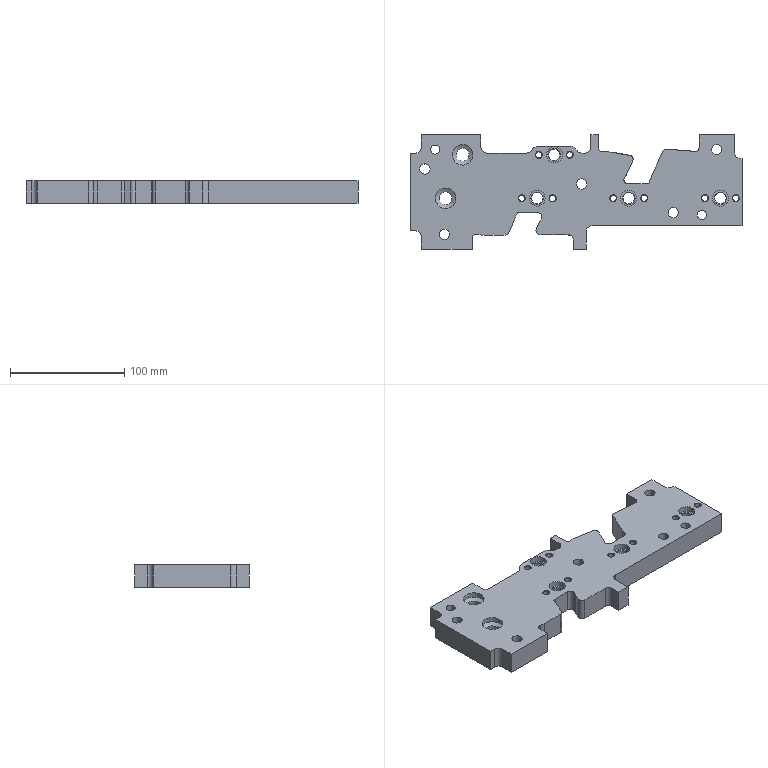Part | CATIA | 1 solid | 166 faces | box 290 x 100 x 19.5 mm | volume 379711 mm3 | cylinder 85 | plane 39 | cone 28 | other 14 | commonest cylinder face diameters 5.2 x16 10 x16 9 x10 15 x10 14 x8 7 x6